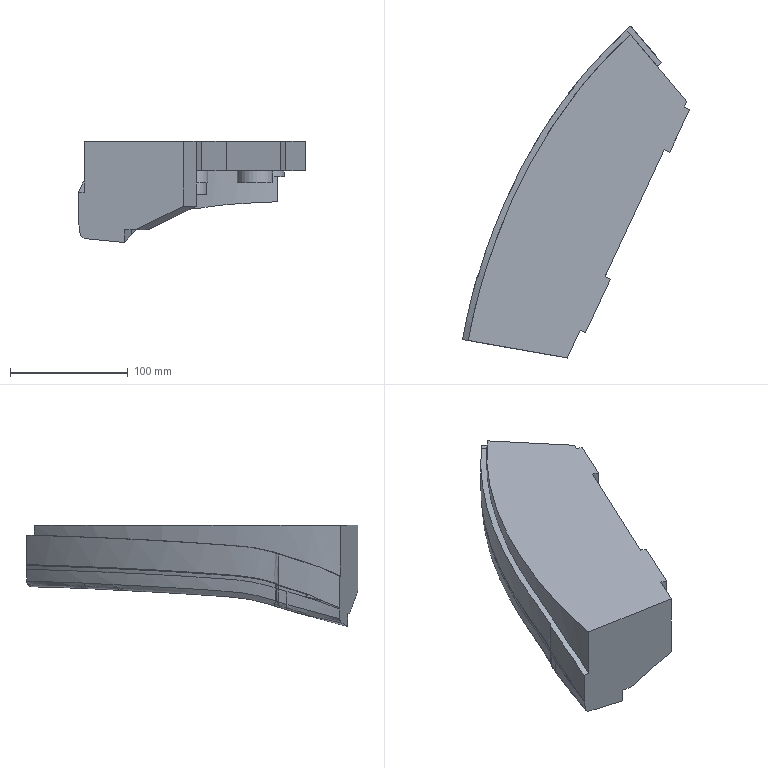Part | NX | features solid 2 | 1 solid | 62 faces | box 193.085 x 282.048 x 86.207 mm | volume 1163833 mm3 | spline 35 | plane 21 | cylinder 6 | commonest cylinder face diameters 30 x4 40 x2